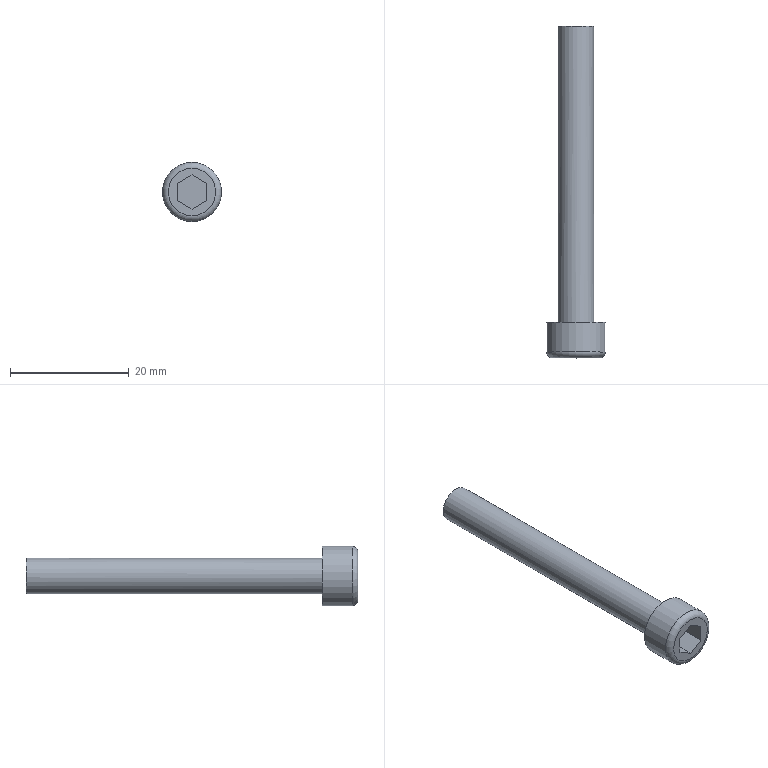Part | STEP file | Tube necking machine_id206_x_t | 1 solid | 13 faces | box 10 x 56 x 10 mm | volume 1793 mm3 | plane 10 | cylinder 2 | torus 1 | commonest cylinder face diameters 6 x1 10 x1
STEP:
#1=CARTESIAN_POINT('',(0.,0.,0.));
#2=DIRECTION('',(0.,0.,1.));
#3=DIRECTION('',(1.,0.,0.));
#4=AXIS2_PLACEMENT_3D('',#1,#2,#3);
#5=CARTESIAN_POINT('',(-115.,-134.,585.));
#6=VERTEX_POINT('',#5);
#7=CARTESIAN_POINT('',(-115.,-134.,581.));
#8=DIRECTION('',(0.,-1.,0.));
#9=DIRECTION('',(0.,0.,1.));
#10=AXIS2_PLACEMENT_3D('',#7,#8,#9);
#11=CIRCLE('',#10,4.);
#12=CARTESIAN_POINT('',(-115.,-134.,576.));
#13=DIRECTION('',(0.,1.,0.));
#14=DIRECTION('',(0.,0.,1.));
#15=AXIS2_PLACEMENT_3D('',#12,#13,#14);
#16=PLANE('',#15);
#17=CARTESIAN_POINT('',(9.,0.));
#18=CARTESIAN_POINT('',(9.,-6.928));
#19=CARTESIAN_POINT('',(3.,-3.464));
#20=CARTESIAN_POINT('',(-3.,0.));
#21=CARTESIAN_POINT('',(3.,3.464));
#22=CARTESIAN_POINT('',(9.,6.928));
#23=CARTESIAN_POINT('',(9.,0.));
#24=(BOUNDED_CURVE()B_SPLINE_CURVE(2,(#17,#18,#19,#20,#21,#22,#23),.UNSPECIFIED.,.T.,.F.)B_SPLINE_CURVE_WITH_KNOTS((1,2,2,2,2,1),(-2.094,0.,2.094,4.189,6.283,8.378),.UNSPECIFIED.)CURVE()GEOMETRIC_REPRESENTATION_ITEM()RATIONAL_B_SPLINE_CURVE((1.,0.5,1.,0.5,1.,0.5,1.))REPRESENTATION_ITEM(''));
#25=(GEOMETRIC_REPRESENTATION_CONTEXT(2)PARAMETRIC_REPRESENTATION_CONTEXT()REPRESENTATION_CONTEXT('',''));
#26=DEFINITIONAL_REPRESENTATION('',(#24),#25);
#27=PCURVE('',#16,#26);
#28=CARTESIAN_POINT('',(-115.,-133.,581.));
#29=DIRECTION('',(0.,1.,0.));
#30=DIRECTION('',(0.,0.,1.));
#31=AXIS2_PLACEMENT_3D('',#28,#29,#30);
#32=TOROIDAL_SURFACE('',#31,4.,1.);
#33=CARTESIAN_POINT('',(6.283,4.712));
#34=DIRECTION('',(-1.,0.));
#35=VECTOR('',#34,1.);
#36=LINE('',#33,#35);
#37=(GEOMETRIC_REPRESENTATION_CONTEXT(2)PARAMETRIC_REPRESENTATION_CONTEXT()REPRESENTATION_CONTEXT('',''));
#38=DEFINITIONAL_REPRESENTATION('',(#36),#37);
#39=PCURVE('',#32,#38);
#40=SURFACE_CURVE('',#11,(#27,#39),.PCURVE_S1.);
#41=EDGE_CURVE('',#6,#6,#40,.T.);
#42=ORIENTED_EDGE('',*,*,#41,.T.);
#43=EDGE_LOOP('',(#42));
#44=FACE_BOUND('',#43,.T.);
#45=CARTESIAN_POINT('',(-117.5,-134.,579.557));
#46=VERTEX_POINT('',#45);
#47=CARTESIAN_POINT('',(-117.5,-134.,582.443));
#48=VERTEX_POINT('',#47);
#49=CARTESIAN_POINT('',(-117.5,-134.,582.443));
#50=DIRECTION('',(0.,0.,1.));
#51=VECTOR('',#50,1.);
#52=LINE('',#49,#51);
#53=CARTESIAN_POINT('',(6.443,-2.5));
#54=DIRECTION('',(1.,0.));
#55=VECTOR('',#54,1.);
#56=LINE('',#53,#55);
#57=(GEOMETRIC_REPRESENTATION_CONTEXT(2)PARAMETRIC_REPRESENTATION_CONTEXT()REPRESENTATION_CONTEXT('',''));
#58=DEFINITIONAL_REPRESENTATION('',(#56),#57);
#59=PCURVE('',#16,#58);
#60=CARTESIAN_POINT('',(-117.5,-130.04,582.443));
#61=DIRECTION('',(1.,0.,0.));
#62=DIRECTION('',(0.,1.,0.));
#63=AXIS2_PLACEMENT_3D('',#60,#61,#62);
#64=PLANE('',#63);
#65=CARTESIAN_POINT('',(-3.96,0.));
#66=DIRECTION('',(0.,1.));
#67=VECTOR('',#66,1.);
#68=LINE('',#65,#67);
#69=(GEOMETRIC_REPRESENTATION_CONTEXT(2)PARAMETRIC_REPRESENTATION_CONTEXT()REPRESENTATION_CONTEXT('',''));
#70=DEFINITIONAL_REPRESENTATION('',(#68),#69);
#71=PCURVE('',#64,#70);
#72=SURFACE_CURVE('',#52,(#59,#71),.PCURVE_S1.);
#73=EDGE_CURVE('',#46,#48,#72,.T.);
#74=ORIENTED_EDGE('',*,*,#73,.T.);
#75=CARTESIAN_POINT('',(-115.,-134.,583.887));
#76=VERTEX_POINT('',#75);
#77=CARTESIAN_POINT('',(-115.,-134.,583.887));
#78=DIRECTION('',(0.866,0.,0.5));
#79=VECTOR('',#78,1.);
#80=LINE('',#77,#79);
#81=CARTESIAN_POINT('',(7.887,0.));
#82=DIRECTION('',(0.5,0.866));
#83=VECTOR('',#82,1.);
#84=LINE('',#81,#83);
#85=(GEOMETRIC_REPRESENTATION_CONTEXT(2)PARAMETRIC_REPRESENTATION_CONTEXT()REPRESENTATION_CONTEXT('',''));
#86=DEFINITIONAL_REPRESENTATION('',(#84),#85);
#87=PCURVE('',#16,#86);
#88=CARTESIAN_POINT('',(-115.,-130.04,583.887));
#89=DIRECTION('',(0.5,0.,-0.866));
#90=DIRECTION('',(-0.866,0.,-0.5));
#91=AXIS2_PLACEMENT_3D('',#88,#89,#90);
#92=PLANE('',#91);
#93=CARTESIAN_POINT('',(0.,-3.96));
#94=DIRECTION('',(-1.,0.));
#95=VECTOR('',#94,1.);
#96=LINE('',#93,#95);
#97=(GEOMETRIC_REPRESENTATION_CONTEXT(2)PARAMETRIC_REPRESENTATION_CONTEXT()REPRESENTATION_CONTEXT('',''));
#98=DEFINITIONAL_REPRESENTATION('',(#96),#97);
#99=PCURVE('',#92,#98);
#100=SURFACE_CURVE('',#80,(#87,#99),.PCURVE_S1.);
#101=EDGE_CURVE('',#48,#76,#100,.T.);
#102=ORIENTED_EDGE('',*,*,#101,.T.);
#103=CARTESIAN_POINT('',(-112.5,-134.,582.443));
#104=VERTEX_POINT('',#103);
#105=CARTESIAN_POINT('',(-112.5,-134.,582.443));
#106=DIRECTION('',(0.866,0.,-0.5));
#107=VECTOR('',#106,1.);
#108=LINE('',#105,#107);
#109=CARTESIAN_POINT('',(6.443,2.5));
#110=DIRECTION('',(-0.5,0.866));
#111=VECTOR('',#110,1.);
#112=LINE('',#109,#111);
#113=(GEOMETRIC_REPRESENTATION_CONTEXT(2)PARAMETRIC_REPRESENTATION_CONTEXT()REPRESENTATION_CONTEXT('',''));
#114=DEFINITIONAL_REPRESENTATION('',(#112),#113);
#115=PCURVE('',#16,#114);
#116=CARTESIAN_POINT('',(-112.5,-130.04,582.443));
#117=DIRECTION('',(-0.5,0.,-0.866));
#118=DIRECTION('',(-0.866,0.,0.5));
#119=AXIS2_PLACEMENT_3D('',#116,#117,#118);
#120=PLANE('',#119);
#121=CARTESIAN_POINT('',(0.,-3.96));
#122=DIRECTION('',(-1.,0.));
#123=VECTOR('',#122,1.);
#124=LINE('',#121,#123);
#125=(GEOMETRIC_REPRESENTATION_CONTEXT(2)PARAMETRIC_REPRESENTATION_CONTEXT()REPRESENTATION_CONTEXT('',''));
#126=DEFINITIONAL_REPRESENTATION('',(#124),#125);
#127=PCURVE('',#120,#126);
#128=SURFACE_CURVE('',#108,(#115,#127),.PCURVE_S1.);
#129=EDGE_CURVE('',#76,#104,#128,.T.);
#130=ORIENTED_EDGE('',*,*,#129,.T.);
#131=CARTESIAN_POINT('',(-112.5,-134.,579.557));
#132=VERTEX_POINT('',#131);
#133=CARTESIAN_POINT('',(-112.5,-134.,579.557));
#134=DIRECTION('',(0.,0.,-1.));
#135=VECTOR('',#134,1.);
#136=LINE('',#133,#135);
#137=CARTESIAN_POINT('',(3.557,2.5));
#138=DIRECTION('',(-1.,0.));
#139=VECTOR('',#138,1.);
#140=LINE('',#137,#139);
#141=(GEOMETRIC_REPRESENTATION_CONTEXT(2)PARAMETRIC_REPRESENTATION_CONTEXT()REPRESENTATION_CONTEXT('',''));
#142=DEFINITIONAL_REPRESENTATION('',(#140),#141);
#143=PCURVE('',#16,#142);
#144=CARTESIAN_POINT('',(-112.5,-130.04,579.557));
#145=DIRECTION('',(-1.,0.,0.));
#146=DIRECTION('',(0.,0.,1.));
#147=AXIS2_PLACEMENT_3D('',#144,#145,#146);
#148=PLANE('',#147);
#149=CARTESIAN_POINT('',(0.,-3.96));
#150=DIRECTION('',(-1.,0.));
#151=VECTOR('',#150,1.);
#152=LINE('',#149,#151);
#153=(GEOMETRIC_REPRESENTATION_CONTEXT(2)PARAMETRIC_REPRESENTATION_CONTEXT()REPRESENTATION_CONTEXT('',''));
#154=DEFINITIONAL_REPRESENTATION('',(#152),#153);
#155=PCURVE('',#148,#154);
#156=SURFACE_CURVE('',#136,(#143,#155),.PCURVE_S1.);
#157=EDGE_CURVE('',#104,#132,#156,.T.);
#158=ORIENTED_EDGE('',*,*,#157,.T.);
#159=CARTESIAN_POINT('',(-115.,-134.,578.113));
#160=VERTEX_POINT('',#159);
#161=CARTESIAN_POINT('',(-115.,-134.,578.113));
#162=DIRECTION('',(-0.866,0.,-0.5));
#163=VECTOR('',#162,1.);
#164=LINE('',#161,#163);
#165=CARTESIAN_POINT('',(2.113,0.));
#166=DIRECTION('',(-0.5,-0.866));
#167=VECTOR('',#166,1.);
#168=LINE('',#165,#167);
#169=(GEOMETRIC_REPRESENTATION_CONTEXT(2)PARAMETRIC_REPRESENTATION_CONTEXT()REPRESENTATION_CONTEXT('',''));
#170=DEFINITIONAL_REPRESENTATION('',(#168),#169);
#171=PCURVE('',#16,#170);
#172=CARTESIAN_POINT('',(-115.,-130.04,578.113));
#173=DIRECTION('',(-0.5,0.,0.866));
#174=DIRECTION('',(0.866,0.,0.5));
#175=AXIS2_PLACEMENT_3D('',#172,#173,#174);
#176=PLANE('',#175);
#177=CARTESIAN_POINT('',(0.,-3.96));
#178=DIRECTION('',(-1.,0.));
#179=VECTOR('',#178,1.);
#180=LINE('',#177,#179);
#181=(GEOMETRIC_REPRESENTATION_CONTEXT(2)PARAMETRIC_REPRESENTATION_CONTEXT()REPRESENTATION_CONTEXT('',''));
#182=DEFINITIONAL_REPRESENTATION('',(#180),#181);
#183=PCURVE('',#176,#182);
#184=SURFACE_CURVE('',#164,(#171,#183),.PCURVE_S1.);
#185=EDGE_CURVE('',#132,#160,#184,.T.);
#186=ORIENTED_EDGE('',*,*,#185,.T.);
#187=CARTESIAN_POINT('',(-117.5,-134.,579.557));
#188=DIRECTION('',(-0.866,0.,0.5));
#189=VECTOR('',#188,1.);
#190=LINE('',#187,#189);
#191=CARTESIAN_POINT('',(3.557,-2.5));
#192=DIRECTION('',(0.5,-0.866));
#193=VECTOR('',#192,1.);
#194=LINE('',#191,#193);
#195=(GEOMETRIC_REPRESENTATION_CONTEXT(2)PARAMETRIC_REPRESENTATION_CONTEXT()REPRESENTATION_CONTEXT('',''));
#196=DEFINITIONAL_REPRESENTATION('',(#194),#195);
#197=PCURVE('',#16,#196);
#198=CARTESIAN_POINT('',(-117.5,-130.04,579.557));
#199=DIRECTION('',(0.5,0.,0.866));
#200=DIRECTION('',(0.866,0.,-0.5));
#201=AXIS2_PLACEMENT_3D('',#198,#199,#200);
#202=PLANE('',#201);
#203=CARTESIAN_POINT('',(0.,-3.96));
#204=DIRECTION('',(-1.,0.));
#205=VECTOR('',#204,1.);
#206=LINE('',#203,#205);
#207=(GEOMETRIC_REPRESENTATION_CONTEXT(2)PARAMETRIC_REPRESENTATION_CONTEXT()REPRESENTATION_CONTEXT('',''));
#208=DEFINITIONAL_REPRESENTATION('',(#206),#207);
#209=PCURVE('',#202,#208);
#210=SURFACE_CURVE('',#190,(#197,#209),.PCURVE_S1.);
#211=EDGE_CURVE('',#160,#46,#210,.T.);
#212=ORIENTED_EDGE('',*,*,#211,.T.);
#213=EDGE_LOOP('',(#74,#102,#130,#158,#186,#212));
#214=FACE_BOUND('',#213,.T.);
#215=ADVANCED_FACE('',(#44,#214),#16,.F.);
#216=CARTESIAN_POINT('',(-115.,-133.,586.));
#217=VERTEX_POINT('',#216);
#218=CARTESIAN_POINT('',(-115.,-133.,576.));
#219=VERTEX_POINT('',#218);
#220=CARTESIAN_POINT('',(-115.,-133.,581.));
#221=DIRECTION('',(0.,1.,0.));
#222=DIRECTION('',(0.,0.,1.));
#223=AXIS2_PLACEMENT_3D('',#220,#221,#222);
#224=CIRCLE('',#223,5.);
#225=CARTESIAN_POINT('',(-115.,-129.1,581.));
#226=DIRECTION('',(0.,-1.,0.));
#227=DIRECTION('',(0.,0.,-1.));
#228=AXIS2_PLACEMENT_3D('',#225,#226,#227);
#229=CYLINDRICAL_SURFACE('',#228,5.);
#230=CARTESIAN_POINT('',(3.142,3.9));
#231=DIRECTION('',(-1.,0.));
#232=VECTOR('',#231,1.);
#233=LINE('',#230,#232);
#234=(GEOMETRIC_REPRESENTATION_CONTEXT(2)PARAMETRIC_REPRESENTATION_CONTEXT()REPRESENTATION_CONTEXT('',''));
#235=DEFINITIONAL_REPRESENTATION('',(#233),#234);
#236=PCURVE('',#229,#235);
#237=CARTESIAN_POINT('',(0.,6.283));
#238=DIRECTION('',(1.,0.));
#239=VECTOR('',#238,1.);
#240=LINE('',#237,#239);
#241=(GEOMETRIC_REPRESENTATION_CONTEXT(2)PARAMETRIC_REPRESENTATION_CONTEXT()REPRESENTATION_CONTEXT('',''));
#242=DEFINITIONAL_REPRESENTATION('',(#240),#241);
#243=PCURVE('',#32,#242);
#244=SURFACE_CURVE('',#224,(#236,#243),.PCURVE_S1.);
#245=EDGE_CURVE('',#217,#219,#244,.T.);
#246=ORIENTED_EDGE('',*,*,#245,.T.);
#247=CARTESIAN_POINT('',(-115.,-128.,576.));
#248=VERTEX_POINT('',#247);
#249=CARTESIAN_POINT('',(-115.,-128.,576.));
#250=CARTESIAN_POINT('',(-115.,-133.,576.));
#251=B_SPLINE_CURVE_WITH_KNOTS('',1,(#249,#250),.UNSPECIFIED.,.F.,.F.,(2,2),(-1.1,3.9),.PIECEWISE_BEZIER_KNOTS.);
#252=CARTESIAN_POINT('',(0.,0.));
#253=DIRECTION('',(0.,1.));
#254=VECTOR('',#253,1.);
#255=LINE('',#252,#254);
#256=(GEOMETRIC_REPRESENTATION_CONTEXT(2)PARAMETRIC_REPRESENTATION_CONTEXT()REPRESENTATION_CONTEXT('',''));
#257=DEFINITIONAL_REPRESENTATION('',(#255),#256);
#258=PCURVE('',#229,#257);
#259=CARTESIAN_POINT('',(6.283,0.));
#260=DIRECTION('',(0.,1.));
#261=VECTOR('',#260,1.);
#262=LINE('',#259,#261);
#263=(GEOMETRIC_REPRESENTATION_CONTEXT(2)PARAMETRIC_REPRESENTATION_CONTEXT()REPRESENTATION_CONTEXT('',''));
#264=DEFINITIONAL_REPRESENTATION('',(#262),#263);
#265=PCURVE('',#229,#264);
#266=SEAM_CURVE('',#251,(#258,#265),.PCURVE_S1.);
#267=EDGE_CURVE('',#248,#219,#266,.T.);
#268=ORIENTED_EDGE('',*,*,#267,.F.);
#269=CARTESIAN_POINT('',(-115.,-128.,581.));
#270=DIRECTION('',(0.,-1.,0.));
#271=DIRECTION('',(0.,0.,-1.));
#272=AXIS2_PLACEMENT_3D('',#269,#270,#271);
#273=CIRCLE('',#272,5.);
#274=CARTESIAN_POINT('',(0.,-1.1));
#275=DIRECTION('',(1.,0.));
#276=VECTOR('',#275,1.);
#277=LINE('',#274,#276);
#278=(GEOMETRIC_REPRESENTATION_CONTEXT(2)PARAMETRIC_REPRESENTATION_CONTEXT()REPRESENTATION_CONTEXT('',''));
#279=DEFINITIONAL_REPRESENTATION('',(#277),#278);
#280=PCURVE('',#229,#279);
#281=CARTESIAN_POINT('',(-115.,-128.,578.));
#282=DIRECTION('',(0.,-1.,0.));
#283=DIRECTION('',(0.,0.,-1.));
#284=AXIS2_PLACEMENT_3D('',#281,#282,#283);
#285=PLANE('',#284);
#286=CARTESIAN_POINT('',(-3.,0.));
#287=DIRECTION('',(1.,0.));
#288=AXIS2_PLACEMENT_2D('',#286,#287);
#289=CIRCLE('',#288,5.);
#290=(GEOMETRIC_REPRESENTATION_CONTEXT(2)PARAMETRIC_REPRESENTATION_CONTEXT()REPRESENTATION_CONTEXT('',''));
#291=DEFINITIONAL_REPRESENTATION('',(#289),#290);
#292=PCURVE('',#285,#291);
#293=SURFACE_CURVE('',#273,(#280,#292),.PCURVE_S1.);
#294=EDGE_CURVE('',#248,#248,#293,.T.);
#295=ORIENTED_EDGE('',*,*,#294,.T.);
#296=ORIENTED_EDGE('',*,*,#267,.T.);
#297=CARTESIAN_POINT('',(-115.,-133.,581.));
#298=DIRECTION('',(0.,1.,0.));
#299=DIRECTION('',(0.,0.,1.));
#300=AXIS2_PLACEMENT_3D('',#297,#298,#299);
#301=CIRCLE('',#300,5.);
#302=CARTESIAN_POINT('',(9.425,3.9));
#303=DIRECTION('',(-1.,0.));
#304=VECTOR('',#303,1.);
#305=LINE('',#302,#304);
#306=(GEOMETRIC_REPRESENTATION_CONTEXT(2)PARAMETRIC_REPRESENTATION_CONTEXT()REPRESENTATION_CONTEXT('',''));
#307=DEFINITIONAL_REPRESENTATION('',(#305),#306);
#308=PCURVE('',#229,#307);
#309=CARTESIAN_POINT('',(0.,6.283));
#310=DIRECTION('',(1.,0.));
#311=VECTOR('',#310,1.);
#312=LINE('',#309,#311);
#313=(GEOMETRIC_REPRESENTATION_CONTEXT(2)PARAMETRIC_REPRESENTATION_CONTEXT()REPRESENTATION_CONTEXT('',''));
#314=DEFINITIONAL_REPRESENTATION('',(#312),#313);
#315=PCURVE('',#32,#314);
#316=SURFACE_CURVE('',#301,(#308,#315),.PCURVE_S1.);
#317=EDGE_CURVE('',#219,#217,#316,.T.);
#318=ORIENTED_EDGE('',*,*,#317,.T.);
#319=EDGE_LOOP('',(#246,#268,#295,#296,#318));
#320=FACE_BOUND('',#319,.T.);
#321=ADVANCED_FACE('',(#320),#229,.T.);
#322=ORIENTED_EDGE('',*,*,#294,.F.);
#323=EDGE_LOOP('',(#322));
#324=FACE_BOUND('',#323,.T.);
#325=CARTESIAN_POINT('',(-115.,-128.,578.));
#326=VERTEX_POINT('',#325);
#327=CARTESIAN_POINT('',(-115.,-128.,581.));
#328=DIRECTION('',(0.,-1.,0.));
#329=DIRECTION('',(0.,0.,-1.));
#330=AXIS2_PLACEMENT_3D('',#327,#328,#329);
#331=CIRCLE('',#330,3.);
#332=CARTESIAN_POINT('',(-3.,0.));
#333=DIRECTION('',(1.,0.));
#334=AXIS2_PLACEMENT_2D('',#332,#333);
#335=CIRCLE('',#334,3.);
#336=(GEOMETRIC_REPRESENTATION_CONTEXT(2)PARAMETRIC_REPRESENTATION_CONTEXT()REPRESENTATION_CONTEXT('',''));
#337=DEFINITIONAL_REPRESENTATION('',(#335),#336);
#338=PCURVE('',#285,#337);
#339=CARTESIAN_POINT('',(-115.,-129.1,581.));
#340=DIRECTION('',(0.,-1.,0.));
#341=DIRECTION('',(0.,0.,-1.));
#342=AXIS2_PLACEMENT_3D('',#339,#340,#341);
#343=CYLINDRICAL_SURFACE('',#342,3.);
#344=CARTESIAN_POINT('',(0.,-1.1));
#345=DIRECTION('',(1.,0.));
#346=VECTOR('',#345,1.);
#347=LINE('',#344,#346);
#348=(GEOMETRIC_REPRESENTATION_CONTEXT(2)PARAMETRIC_REPRESENTATION_CONTEXT()REPRESENTATION_CONTEXT('',''));
#349=DEFINITIONAL_REPRESENTATION('',(#347),#348);
#350=PCURVE('',#343,#349);
#351=SURFACE_CURVE('',#331,(#338,#350),.PCURVE_S1.);
#352=EDGE_CURVE('',#326,#326,#351,.T.);
#353=ORIENTED_EDGE('',*,*,#352,.T.);
#354=EDGE_LOOP('',(#353));
#355=FACE_BOUND('',#354,.T.);
#356=ADVANCED_FACE('',(#324,#355),#285,.F.);
#357=ORIENTED_EDGE('',*,*,#352,.F.);
#358=CARTESIAN_POINT('',(-115.,-78.,578.));
#359=VERTEX_POINT('',#358);
#360=CARTESIAN_POINT('',(-115.,-78.,578.));
#361=CARTESIAN_POINT('',(-115.,-128.,578.));
#362=B_SPLINE_CURVE_WITH_KNOTS('',1,(#360,#361),.UNSPECIFIED.,.F.,.F.,(2,2),(-51.1,-1.1),.PIECEWISE_BEZIER_KNOTS.);
#363=CARTESIAN_POINT('',(0.,0.));
#364=DIRECTION('',(0.,1.));
#365=VECTOR('',#364,1.);
#366=LINE('',#363,#365);
#367=(GEOMETRIC_REPRESENTATION_CONTEXT(2)PARAMETRIC_REPRESENTATION_CONTEXT()REPRESENTATION_CONTEXT('',''));
#368=DEFINITIONAL_REPRESENTATION('',(#366),#367);
#369=PCURVE('',#343,#368);
#370=CARTESIAN_POINT('',(6.283,0.));
#371=DIRECTION('',(0.,1.));
#372=VECTOR('',#371,1.);
#373=LINE('',#370,#372);
#374=(GEOMETRIC_REPRESENTATION_CONTEXT(2)PARAMETRIC_REPRESENTATION_CONTEXT()REPRESENTATION_CONTEXT('',''));
#375=DEFINITIONAL_REPRESENTATION('',(#373),#374);
#376=PCURVE('',#343,#375);
#377=SEAM_CURVE('',#362,(#369,#376),.PCURVE_S1.);
#378=EDGE_CURVE('',#359,#326,#377,.T.);
#379=ORIENTED_EDGE('',*,*,#378,.F.);
#380=CARTESIAN_POINT('',(-112.,-78.,581.));
#381=VERTEX_POINT('',#380);
#382=CARTESIAN_POINT('',(-115.,-78.,581.));
#383=DIRECTION('',(0.,-1.,0.));
#384=DIRECTION('',(1.,0.,0.));
#385=AXIS2_PLACEMENT_3D('',#382,#383,#384);
#386=CIRCLE('',#385,3.);
#387=CARTESIAN_POINT('',(-4.712,-51.1));
#388=DIRECTION('',(1.,0.));
#389=VECTOR('',#388,1.);
#390=LINE('',#387,#389);
#391=(GEOMETRIC_REPRESENTATION_CONTEXT(2)PARAMETRIC_REPRESENTATION_CONTEXT()REPRESENTATION_CONTEXT('',''));
#392=DEFINITIONAL_REPRESENTATION('',(#390),#391);
#393=PCURVE('',#343,#392);
#394=CARTESIAN_POINT('',(-92.5,-78.,191.));
#395=DIRECTION('',(0.,1.,0.));
#396=DIRECTION('',(-1.,0.,0.));
#397=AXIS2_PLACEMENT_3D('',#394,#395,#396);
#398=PLANE('',#397);
#399=CARTESIAN_POINT('',(19.5,390.));
#400=CARTESIAN_POINT('',(19.5,395.196));
#401=CARTESIAN_POINT('',(24.,392.598));
#402=CARTESIAN_POINT('',(28.5,390.));
#403=CARTESIAN_POINT('',(24.,387.402));
#404=CARTESIAN_POINT('',(19.5,384.804));
#405=CARTESIAN_POINT('',(19.5,390.));
#406=(BOUNDED_CURVE()B_SPLINE_CURVE(2,(#399,#400,#401,#402,#403,#404,#405),.UNSPECIFIED.,.T.,.F.)B_SPLINE_CURVE_WITH_KNOTS((1,2,2,2,2,1),(-2.094,0.,2.094,4.189,6.283,8.378),.UNSPECIFIED.)CURVE()GEOMETRIC_REPRESENTATION_ITEM()RATIONAL_B_SPLINE_CURVE((1.,0.5,1.,0.5,1.,0.5,1.))REPRESENTATION_ITEM(''));
#407=(GEOMETRIC_REPRESENTATION_CONTEXT(2)PARAMETRIC_REPRESENTATION_CONTEXT()REPRESENTATION_CONTEXT('',''));
#408=DEFINITIONAL_REPRESENTATION('',(#406),#407);
#409=PCURVE('',#398,#408);
#410=SURFACE_CURVE('',#386,(#393,#409),.PCURVE_S1.);
#411=EDGE_CURVE('',#359,#381,#410,.T.);
#412=ORIENTED_EDGE('',*,*,#411,.T.);
#413=CARTESIAN_POINT('',(-115.,-78.,581.));
#414=DIRECTION('',(0.,-1.,0.));
#415=DIRECTION('',(1.,0.,0.));
#416=AXIS2_PLACEMENT_3D('',#413,#414,#415);
#417=CIRCLE('',#416,3.);
#418=CARTESIAN_POINT('',(1.571,-51.1));
#419=DIRECTION('',(1.,0.));
#420=VECTOR('',#419,1.);
#421=LINE('',#418,#420);
#422=(GEOMETRIC_REPRESENTATION_CONTEXT(2)PARAMETRIC_REPRESENTATION_CONTEXT()REPRESENTATION_CONTEXT('',''));
#423=DEFINITIONAL_REPRESENTATION('',(#421),#422);
#424=PCURVE('',#343,#423);
#425=CARTESIAN_POINT('',(19.5,390.));
#426=CARTESIAN_POINT('',(19.5,395.196));
#427=CARTESIAN_POINT('',(24.,392.598));
#428=CARTESIAN_POINT('',(28.5,390.));
#429=CARTESIAN_POINT('',(24.,387.402));
#430=CARTESIAN_POINT('',(19.5,384.804));
#431=CARTESIAN_POINT('',(19.5,390.));
#432=(BOUNDED_CURVE()B_SPLINE_CURVE(2,(#425,#426,#427,#428,#429,#430,#431),.UNSPECIFIED.,.T.,.F.)B_SPLINE_CURVE_WITH_KNOTS((1,2,2,2,2,1),(-2.094,0.,2.094,4.189,6.283,8.378),.UNSPECIFIED.)CURVE()GEOMETRIC_REPRESENTATION_ITEM()RATIONAL_B_SPLINE_CURVE((1.,0.5,1.,0.5,1.,0.5,1.))REPRESENTATION_ITEM(''));
#433=(GEOMETRIC_REPRESENTATION_CONTEXT(2)PARAMETRIC_REPRESENTATION_CONTEXT()REPRESENTATION_CONTEXT('',''));
#434=DEFINITIONAL_REPRESENTATION('',(#432),#433);
#435=PCURVE('',#398,#434);
#436=SURFACE_CURVE('',#417,(#424,#435),.PCURVE_S1.);
#437=EDGE_CURVE('',#381,#359,#436,.T.);
#438=ORIENTED_EDGE('',*,*,#437,.T.);
#439=ORIENTED_EDGE('',*,*,#378,.T.);
#440=EDGE_LOOP('',(#357,#379,#412,#438,#439));
#441=FACE_BOUND('',#440,.T.);
#442=ADVANCED_FACE('',(#441),#343,.T.);
#443=ORIENTED_EDGE('',*,*,#437,.F.);
#444=ORIENTED_EDGE('',*,*,#411,.F.);
#445=EDGE_LOOP('',(#443,#444));
#446=FACE_BOUND('',#445,.T.);
#447=ADVANCED_FACE('',(#446),#398,.T.);
#448=ORIENTED_EDGE('',*,*,#73,.F.);
#449=CARTESIAN_POINT('',(-117.5,-130.04,579.557));
#450=VERTEX_POINT('',#449);
#451=CARTESIAN_POINT('',(-117.5,-130.04,579.557));
#452=DIRECTION('',(0.,-1.,0.));
#453=VECTOR('',#452,1.);
#454=LINE('',#451,#453);
#455=CARTESIAN_POINT('',(0.,-2.887));
#456=DIRECTION('',(-1.,0.));
#457=VECTOR('',#456,1.);
#458=LINE('',#455,#457);
#459=(GEOMETRIC_REPRESENTATION_CONTEXT(2)PARAMETRIC_REPRESENTATION_CONTEXT()REPRESENTATION_CONTEXT('',''));
#460=DEFINITIONAL_REPRESENTATION('',(#458),#459);
#461=PCURVE('',#64,#460);
#462=CARTESIAN_POINT('',(0.,0.));
#463=DIRECTION('',(0.,-1.));
#464=VECTOR('',#463,1.);
#465=LINE('',#462,#464);
#466=(GEOMETRIC_REPRESENTATION_CONTEXT(2)PARAMETRIC_REPRESENTATION_CONTEXT()REPRESENTATION_CONTEXT('',''));
#467=DEFINITIONAL_REPRESENTATION('',(#465),#466);
#468=PCURVE('',#202,#467);
#469=SURFACE_CURVE('',#454,(#461,#468),.PCURVE_S1.);
#470=EDGE_CURVE('',#450,#46,#469,.T.);
#471=ORIENTED_EDGE('',*,*,#470,.F.);
#472=CARTESIAN_POINT('',(-117.5,-130.04,582.443));
#473=VERTEX_POINT('',#472);
#474=CARTESIAN_POINT('',(-117.5,-130.04,582.443));
#475=DIRECTION('',(0.,0.,-1.));
#476=VECTOR('',#475,1.);
#477=LINE('',#474,#476);
#478=CARTESIAN_POINT('',(0.,0.));
#479=DIRECTION('',(0.,-1.));
#480=VECTOR('',#479,1.);
#481=LINE('',#478,#480);
#482=(GEOMETRIC_REPRESENTATION_CONTEXT(2)PARAMETRIC_REPRESENTATION_CONTEXT()REPRESENTATION_CONTEXT('',''));
#483=DEFINITIONAL_REPRESENTATION('',(#481),#482);
#484=PCURVE('',#64,#483);
#485=CARTESIAN_POINT('',(-115.,-130.04,581.));
#486=DIRECTION('',(0.,1.,0.));
#487=DIRECTION('',(0.,0.,1.));
#488=AXIS2_PLACEMENT_3D('',#485,#486,#487);
#489=PLANE('',#488);
#490=CARTESIAN_POINT('',(1.443,-2.5));
#491=DIRECTION('',(-1.,0.));
#492=VECTOR('',#491,1.);
#493=LINE('',#490,#492);
#494=(GEOMETRIC_REPRESENTATION_CONTEXT(2)PARAMETRIC_REPRESENTATION_CONTEXT()REPRESENTATION_CONTEXT('',''));
#495=DEFINITIONAL_REPRESENTATION('',(#493),#494);
#496=PCURVE('',#489,#495);
#497=SURFACE_CURVE('',#477,(#484,#496),.PCURVE_S1.);
#498=EDGE_CURVE('',#473,#450,#497,.T.);
#499=ORIENTED_EDGE('',*,*,#498,.F.);
#500=CARTESIAN_POINT('',(-117.5,-130.04,582.443));
#501=DIRECTION('',(0.,-1.,0.));
#502=VECTOR('',#501,1.);
#503=LINE('',#500,#502);
#504=CARTESIAN_POINT('',(0.,0.));
#505=DIRECTION('',(-1.,0.));
#506=VECTOR('',#505,1.);
#507=LINE('',#504,#506);
#508=(GEOMETRIC_REPRESENTATION_CONTEXT(2)PARAMETRIC_REPRESENTATION_CONTEXT()REPRESENTATION_CONTEXT('',''));
#509=DEFINITIONAL_REPRESENTATION('',(#507),#508);
#510=PCURVE('',#64,#509);
#511=CARTESIAN_POINT('',(2.887,0.));
#512=DIRECTION('',(0.,-1.));
#513=VECTOR('',#512,1.);
#514=LINE('',#511,#513);
#515=(GEOMETRIC_REPRESENTATION_CONTEXT(2)PARAMETRIC_REPRESENTATION_CONTEXT()REPRESENTATION_CONTEXT('',''));
#516=DEFINITIONAL_REPRESENTATION('',(#514),#515);
#517=PCURVE('',#92,#516);
#518=SURFACE_CURVE('',#503,(#510,#517),.PCURVE_S1.);
#519=EDGE_CURVE('',#473,#48,#518,.T.);
#520=ORIENTED_EDGE('',*,*,#519,.T.);
#521=EDGE_LOOP('',(#448,#471,#499,#520));
#522=FACE_BOUND('',#521,.T.);
#523=ADVANCED_FACE('',(#522),#64,.T.);
#524=ORIENTED_EDGE('',*,*,#211,.F.);
#525=CARTESIAN_POINT('',(-115.,-130.04,578.113));
#526=VERTEX_POINT('',#525);
#527=CARTESIAN_POINT('',(-115.,-130.04,578.113));
#528=DIRECTION('',(0.,-1.,0.));
#529=VECTOR('',#528,1.);
#530=LINE('',#527,#529);
#531=CARTESIAN_POINT('',(2.887,0.));
#532=DIRECTION('',(0.,-1.));
#533=VECTOR('',#532,1.);
#534=LINE('',#531,#533);
#535=(GEOMETRIC_REPRESENTATION_CONTEXT(2)PARAMETRIC_REPRESENTATION_CONTEXT()REPRESENTATION_CONTEXT('',''));
#536=DEFINITIONAL_REPRESENTATION('',(#534),#535);
#537=PCURVE('',#202,#536);
#538=CARTESIAN_POINT('',(0.,0.));
#539=DIRECTION('',(0.,-1.));
#540=VECTOR('',#539,1.);
#541=LINE('',#538,#540);
#542=(GEOMETRIC_REPRESENTATION_CONTEXT(2)PARAMETRIC_REPRESENTATION_CONTEXT()REPRESENTATION_CONTEXT('',''));
#543=DEFINITIONAL_REPRESENTATION('',(#541),#542);
#544=PCURVE('',#176,#543);
#545=SURFACE_CURVE('',#530,(#537,#544),.PCURVE_S1.);
#546=EDGE_CURVE('',#526,#160,#545,.T.);
#547=ORIENTED_EDGE('',*,*,#546,.F.);
#548=CARTESIAN_POINT('',(-117.5,-130.04,579.557));
#549=DIRECTION('',(0.866,0.,-0.5));
#550=VECTOR('',#549,1.);
#551=LINE('',#548,#550);
#552=CARTESIAN_POINT('',(0.,0.));
#553=DIRECTION('',(1.,0.));
#554=VECTOR('',#553,1.);
#555=LINE('',#552,#554);
#556=(GEOMETRIC_REPRESENTATION_CONTEXT(2)PARAMETRIC_REPRESENTATION_CONTEXT()REPRESENTATION_CONTEXT('',''));
#557=DEFINITIONAL_REPRESENTATION('',(#555),#556);
#558=PCURVE('',#202,#557);
#559=CARTESIAN_POINT('',(-1.443,-2.5));
#560=DIRECTION('',(-0.5,0.866));
#561=VECTOR('',#560,1.);
#562=LINE('',#559,#561);
#563=(GEOMETRIC_REPRESENTATION_CONTEXT(2)PARAMETRIC_REPRESENTATION_CONTEXT()REPRESENTATION_CONTEXT('',''));
#564=DEFINITIONAL_REPRESENTATION('',(#562),#563);
#565=PCURVE('',#489,#564);
#566=SURFACE_CURVE('',#551,(#558,#565),.PCURVE_S1.);
#567=EDGE_CURVE('',#450,#526,#566,.T.);
#568=ORIENTED_EDGE('',*,*,#567,.F.);
#569=ORIENTED_EDGE('',*,*,#470,.T.);
#570=EDGE_LOOP('',(#524,#547,#568,#569));
#571=FACE_BOUND('',#570,.T.);
#572=ADVANCED_FACE('',(#571),#202,.T.);
#573=ORIENTED_EDGE('',*,*,#185,.F.);
#574=CARTESIAN_POINT('',(-112.5,-130.04,579.557));
#575=VERTEX_POINT('',#574);
#576=CARTESIAN_POINT('',(-112.5,-130.04,579.557));
#577=DIRECTION('',(0.,-1.,0.));
#578=VECTOR('',#577,1.);
#579=LINE('',#576,#578);
#580=CARTESIAN_POINT('',(2.887,0.));
#581=DIRECTION('',(0.,-1.));
#582=VECTOR('',#581,1.);
#583=LINE('',#580,#582);
#584=(GEOMETRIC_REPRESENTATION_CONTEXT(2)PARAMETRIC_REPRESENTATION_CONTEXT()REPRESENTATION_CONTEXT('',''));
#585=DEFINITIONAL_REPRESENTATION('',(#583),#584);
#586=PCURVE('',#176,#585);
#587=CARTESIAN_POINT('',(0.,0.));
#588=DIRECTION('',(0.,-1.));
#589=VECTOR('',#588,1.);
#590=LINE('',#587,#589);
#591=(GEOMETRIC_REPRESENTATION_CONTEXT(2)PARAMETRIC_REPRESENTATION_CONTEXT()REPRESENTATION_CONTEXT('',''));
#592=DEFINITIONAL_REPRESENTATION('',(#590),#591);
#593=PCURVE('',#148,#592);
#594=SURFACE_CURVE('',#579,(#586,#593),.PCURVE_S1.);
#595=EDGE_CURVE('',#575,#132,#594,.T.);
#596=ORIENTED_EDGE('',*,*,#595,.F.);
#597=CARTESIAN_POINT('',(-115.,-130.04,578.113));
#598=DIRECTION('',(0.866,0.,0.5));
#599=VECTOR('',#598,1.);
#600=LINE('',#597,#599);
#601=CARTESIAN_POINT('',(0.,0.));
#602=DIRECTION('',(1.,0.));
#603=VECTOR('',#602,1.);
#604=LINE('',#601,#603);
#605=(GEOMETRIC_REPRESENTATION_CONTEXT(2)PARAMETRIC_REPRESENTATION_CONTEXT()REPRESENTATION_CONTEXT('',''));
#606=DEFINITIONAL_REPRESENTATION('',(#604),#605);
#607=PCURVE('',#176,#606);
#608=CARTESIAN_POINT('',(-2.887,0.));
#609=DIRECTION('',(0.5,0.866));
#610=VECTOR('',#609,1.);
#611=LINE('',#608,#610);
#612=(GEOMETRIC_REPRESENTATION_CONTEXT(2)PARAMETRIC_REPRESENTATION_CONTEXT()REPRESENTATION_CONTEXT('',''));
#613=DEFINITIONAL_REPRESENTATION('',(#611),#612);
#614=PCURVE('',#489,#613);
#615=SURFACE_CURVE('',#600,(#607,#614),.PCURVE_S1.);
#616=EDGE_CURVE('',#526,#575,#615,.T.);
#617=ORIENTED_EDGE('',*,*,#616,.F.);
#618=ORIENTED_EDGE('',*,*,#546,.T.);
#619=EDGE_LOOP('',(#573,#596,#617,#618));
#620=FACE_BOUND('',#619,.T.);
#621=ADVANCED_FACE('',(#620),#176,.T.);
#622=ORIENTED_EDGE('',*,*,#157,.F.);
#623=CARTESIAN_POINT('',(-112.5,-130.04,582.443));
#624=VERTEX_POINT('',#623);
#625=CARTESIAN_POINT('',(-112.5,-130.04,582.443));
#626=DIRECTION('',(0.,-1.,0.));
#627=VECTOR('',#626,1.);
#628=LINE('',#625,#627);
#629=CARTESIAN_POINT('',(2.887,0.));
#630=DIRECTION('',(0.,-1.));
#631=VECTOR('',#630,1.);
#632=LINE('',#629,#631);
#633=(GEOMETRIC_REPRESENTATION_CONTEXT(2)PARAMETRIC_REPRESENTATION_CONTEXT()REPRESENTATION_CONTEXT('',''));
#634=DEFINITIONAL_REPRESENTATION('',(#632),#633);
#635=PCURVE('',#148,#634);
#636=CARTESIAN_POINT('',(0.,0.));
#637=DIRECTION('',(0.,-1.));
#638=VECTOR('',#637,1.);
#639=LINE('',#636,#638);
#640=(GEOMETRIC_REPRESENTATION_CONTEXT(2)PARAMETRIC_REPRESENTATION_CONTEXT()REPRESENTATION_CONTEXT('',''));
#641=DEFINITIONAL_REPRESENTATION('',(#639),#640);
#642=PCURVE('',#120,#641);
#643=SURFACE_CURVE('',#628,(#635,#642),.PCURVE_S1.);
#644=EDGE_CURVE('',#624,#104,#643,.T.);
#645=ORIENTED_EDGE('',*,*,#644,.F.);
#646=CARTESIAN_POINT('',(-112.5,-130.04,579.557));
#647=DIRECTION('',(0.,0.,1.));
#648=VECTOR('',#647,1.);
#649=LINE('',#646,#648);
#650=CARTESIAN_POINT('',(0.,0.));
#651=DIRECTION('',(1.,0.));
#652=VECTOR('',#651,1.);
#653=LINE('',#650,#652);
#654=(GEOMETRIC_REPRESENTATION_CONTEXT(2)PARAMETRIC_REPRESENTATION_CONTEXT()REPRESENTATION_CONTEXT('',''));
#655=DEFINITIONAL_REPRESENTATION('',(#653),#654);
#656=PCURVE('',#148,#655);
#657=CARTESIAN_POINT('',(-1.443,2.5));
#658=DIRECTION('',(1.,0.));
#659=VECTOR('',#658,1.);
#660=LINE('',#657,#659);
#661=(GEOMETRIC_REPRESENTATION_CONTEXT(2)PARAMETRIC_REPRESENTATION_CONTEXT()REPRESENTATION_CONTEXT('',''));
#662=DEFINITIONAL_REPRESENTATION('',(#660),#661);
#663=PCURVE('',#489,#662);
#664=SURFACE_CURVE('',#649,(#656,#663),.PCURVE_S1.);
#665=EDGE_CURVE('',#575,#624,#664,.T.);
#666=ORIENTED_EDGE('',*,*,#665,.F.);
#667=ORIENTED_EDGE('',*,*,#595,.T.);
#668=EDGE_LOOP('',(#622,#645,#666,#667));
#669=FACE_BOUND('',#668,.T.);
#670=ADVANCED_FACE('',(#669),#148,.T.);
#671=ORIENTED_EDGE('',*,*,#129,.F.);
#672=CARTESIAN_POINT('',(-115.,-130.04,583.887));
#673=VERTEX_POINT('',#672);
#674=CARTESIAN_POINT('',(-115.,-130.04,583.887));
#675=DIRECTION('',(0.,-1.,0.));
#676=VECTOR('',#675,1.);
#677=LINE('',#674,#676);
#678=CARTESIAN_POINT('',(2.887,0.));
#679=DIRECTION('',(0.,-1.));
#680=VECTOR('',#679,1.);
#681=LINE('',#678,#680);
#682=(GEOMETRIC_REPRESENTATION_CONTEXT(2)PARAMETRIC_REPRESENTATION_CONTEXT()REPRESENTATION_CONTEXT('',''));
#683=DEFINITIONAL_REPRESENTATION('',(#681),#682);
#684=PCURVE('',#120,#683);
#685=CARTESIAN_POINT('',(0.,0.));
#686=DIRECTION('',(0.,-1.));
#687=VECTOR('',#686,1.);
#688=LINE('',#685,#687);
#689=(GEOMETRIC_REPRESENTATION_CONTEXT(2)PARAMETRIC_REPRESENTATION_CONTEXT()REPRESENTATION_CONTEXT('',''));
#690=DEFINITIONAL_REPRESENTATION('',(#688),#689);
#691=PCURVE('',#92,#690);
#692=SURFACE_CURVE('',#677,(#684,#691),.PCURVE_S1.);
#693=EDGE_CURVE('',#673,#76,#692,.T.);
#694=ORIENTED_EDGE('',*,*,#693,.F.);
#695=CARTESIAN_POINT('',(-112.5,-130.04,582.443));
#696=DIRECTION('',(-0.866,0.,0.5));
#697=VECTOR('',#696,1.);
#698=LINE('',#695,#697);
#699=CARTESIAN_POINT('',(0.,0.));
#700=DIRECTION('',(1.,0.));
#701=VECTOR('',#700,1.);
#702=LINE('',#699,#701);
#703=(GEOMETRIC_REPRESENTATION_CONTEXT(2)PARAMETRIC_REPRESENTATION_CONTEXT()REPRESENTATION_CONTEXT('',''));
#704=DEFINITIONAL_REPRESENTATION('',(#702),#703);
#705=PCURVE('',#120,#704);
#706=CARTESIAN_POINT('',(1.443,2.5));
#707=DIRECTION('',(0.5,-0.866));
#708=VECTOR('',#707,1.);
#709=LINE('',#706,#708);
#710=(GEOMETRIC_REPRESENTATION_CONTEXT(2)PARAMETRIC_REPRESENTATION_CONTEXT()REPRESENTATION_CONTEXT('',''));
#711=DEFINITIONAL_REPRESENTATION('',(#709),#710);
#712=PCURVE('',#489,#711);
#713=SURFACE_CURVE('',#698,(#705,#712),.PCURVE_S1.);
#714=EDGE_CURVE('',#624,#673,#713,.T.);
#715=ORIENTED_EDGE('',*,*,#714,.F.);
#716=ORIENTED_EDGE('',*,*,#644,.T.);
#717=EDGE_LOOP('',(#671,#694,#715,#716));
#718=FACE_BOUND('',#717,.T.);
#719=ADVANCED_FACE('',(#718),#120,.T.);
#720=ORIENTED_EDGE('',*,*,#101,.F.);
#721=ORIENTED_EDGE('',*,*,#519,.F.);
#722=CARTESIAN_POINT('',(-115.,-130.04,583.887));
#723=DIRECTION('',(-0.866,0.,-0.5));
#724=VECTOR('',#723,1.);
#725=LINE('',#722,#724);
#726=CARTESIAN_POINT('',(0.,0.));
#727=DIRECTION('',(1.,0.));
#728=VECTOR('',#727,1.);
#729=LINE('',#726,#728);
#730=(GEOMETRIC_REPRESENTATION_CONTEXT(2)PARAMETRIC_REPRESENTATION_CONTEXT()REPRESENTATION_CONTEXT('',''));
#731=DEFINITIONAL_REPRESENTATION('',(#729),#730);
#732=PCURVE('',#92,#731);
#733=CARTESIAN_POINT('',(2.887,0.));
#734=DIRECTION('',(-0.5,-0.866));
#735=VECTOR('',#734,1.);
#736=LINE('',#733,#735);
#737=(GEOMETRIC_REPRESENTATION_CONTEXT(2)PARAMETRIC_REPRESENTATION_CONTEXT()REPRESENTATION_CONTEXT('',''));
#738=DEFINITIONAL_REPRESENTATION('',(#736),#737);
#739=PCURVE('',#489,#738);
#740=SURFACE_CURVE('',#725,(#732,#739),.PCURVE_S1.);
#741=EDGE_CURVE('',#673,#473,#740,.T.);
#742=ORIENTED_EDGE('',*,*,#741,.F.);
#743=ORIENTED_EDGE('',*,*,#693,.T.);
#744=EDGE_LOOP('',(#720,#721,#742,#743));
#745=FACE_BOUND('',#744,.T.);
#746=ADVANCED_FACE('',(#745),#92,.T.);
#747=ORIENTED_EDGE('',*,*,#498,.T.);
#748=ORIENTED_EDGE('',*,*,#567,.T.);
#749=ORIENTED_EDGE('',*,*,#616,.T.);
#750=ORIENTED_EDGE('',*,*,#665,.T.);
#751=ORIENTED_EDGE('',*,*,#714,.T.);
#752=ORIENTED_EDGE('',*,*,#741,.T.);
#753=EDGE_LOOP('',(#747,#748,#749,#750,#751,#752));
#754=FACE_BOUND('',#753,.T.);
#755=ADVANCED_FACE('',(#754),#489,.F.);
#756=ORIENTED_EDGE('',*,*,#245,.F.);
#757=CARTESIAN_POINT('',(-115.,-134.,585.));
#758=CARTESIAN_POINT('',(-115.,-134.,585.267));
#759=CARTESIAN_POINT('',(-115.,-133.915,585.528));
#760=CARTESIAN_POINT('',(-115.,-133.752,585.752));
#761=CARTESIAN_POINT('',(-115.,-133.528,585.915));
#762=CARTESIAN_POINT('',(-115.,-133.267,586.));
#763=CARTESIAN_POINT('',(-115.,-133.,586.));
#764=(BOUNDED_CURVE()B_SPLINE_CURVE(6,(#757,#758,#759,#760,#761,#762,#763),.UNSPECIFIED.,.F.,.F.)B_SPLINE_CURVE_WITH_KNOTS((7,7),(-1.571,0.),.PIECEWISE_BEZIER_KNOTS.)CURVE()GEOMETRIC_REPRESENTATION_ITEM()RATIONAL_B_SPLINE_CURVE((1.031,1.01,0.9979,0.994,0.9979,1.01,1.031))REPRESENTATION_ITEM(''));
#765=CARTESIAN_POINT('',(0.,6.283));
#766=DIRECTION('',(0.,1.));
#767=VECTOR('',#766,1.);
#768=LINE('',#765,#767);
#769=(GEOMETRIC_REPRESENTATION_CONTEXT(2)PARAMETRIC_REPRESENTATION_CONTEXT()REPRESENTATION_CONTEXT('',''));
#770=DEFINITIONAL_REPRESENTATION('',(#768),#769);
#771=PCURVE('',#32,#770);
#772=CARTESIAN_POINT('',(6.283,6.283));
#773=DIRECTION('',(0.,1.));
#774=VECTOR('',#773,1.);
#775=LINE('',#772,#774);
#776=(GEOMETRIC_REPRESENTATION_CONTEXT(2)PARAMETRIC_REPRESENTATION_CONTEXT()REPRESENTATION_CONTEXT('',''));
#777=DEFINITIONAL_REPRESENTATION('',(#775),#776);
#778=PCURVE('',#32,#777);
#779=SEAM_CURVE('',#764,(#771,#778),.PCURVE_S1.);
#780=EDGE_CURVE('',#6,#217,#779,.T.);
#781=ORIENTED_EDGE('',*,*,#780,.F.);
#782=ORIENTED_EDGE('',*,*,#41,.F.);
#783=ORIENTED_EDGE('',*,*,#780,.T.);
#784=ORIENTED_EDGE('',*,*,#317,.F.);
#785=EDGE_LOOP('',(#756,#781,#782,#783,#784));
#786=FACE_BOUND('',#785,.T.);
#787=ADVANCED_FACE('',(#786),#32,.T.);
#788=CLOSED_SHELL('',(#215,#321,#356,#442,#447,#523,#572,#621,#670,#719,#746,#755,#787));
#789=MANIFOLD_SOLID_BREP('',#788);
#790=(LENGTH_UNIT()NAMED_UNIT(*)SI_UNIT(.MILLI.,.METRE.));
#791=UNCERTAINTY_MEASURE_WITH_UNIT(LENGTH_MEASURE(0.000002),#790,'','');
#792=(NAMED_UNIT(*)PLANE_ANGLE_UNIT()SI_UNIT($,.RADIAN.));
#793=(NAMED_UNIT(*)SI_UNIT($,.STERADIAN.)SOLID_ANGLE_UNIT());
#794=(GEOMETRIC_REPRESENTATION_CONTEXT(3)GLOBAL_UNCERTAINTY_ASSIGNED_CONTEXT((#791))GLOBAL_UNIT_ASSIGNED_CONTEXT((#790,#792,#793))REPRESENTATION_CONTEXT('',''));
#795=ADVANCED_BREP_SHAPE_REPRESENTATION('',(#4,#789),#794);